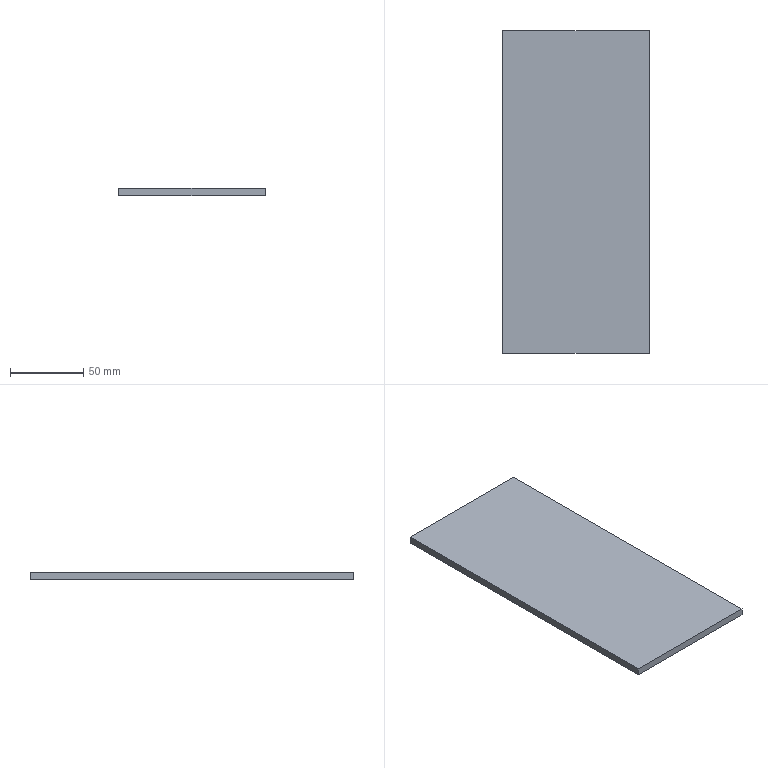Part | SolidWorks | features Extrusion 1 | 1 solid | 6 faces | box 100 x 220 x 5 mm | volume 110000 mm3 | plane 6
STEP:
#1=CARTESIAN_POINT('',(50.,-110.,0.));
#2=VERTEX_POINT('',#1);
#3=CARTESIAN_POINT('',(50.,110.,0.));
#4=VERTEX_POINT('',#3);
#5=CARTESIAN_POINT('',(50.,110.,0.));
#6=DIRECTION('',(0.,1.,0.));
#7=VECTOR('',#6,1000.);
#8=LINE('',#5,#7);
#9=EDGE_CURVE('',#2,#4,#8,.T.);
#10=ORIENTED_EDGE('',*,*,#9,.T.);
#11=CARTESIAN_POINT('',(50.,110.,5.));
#12=VERTEX_POINT('',#11);
#13=CARTESIAN_POINT('',(50.,110.,5.));
#14=DIRECTION('',(0.,0.,-1.));
#15=VECTOR('',#14,1000.);
#16=LINE('',#13,#15);
#17=EDGE_CURVE('',#12,#4,#16,.T.);
#18=ORIENTED_EDGE('',*,*,#17,.F.);
#19=CARTESIAN_POINT('',(50.,-110.,5.));
#20=VERTEX_POINT('',#19);
#21=CARTESIAN_POINT('',(50.,110.,5.));
#22=DIRECTION('',(0.,1.,0.));
#23=VECTOR('',#22,1000.);
#24=LINE('',#21,#23);
#25=EDGE_CURVE('',#20,#12,#24,.T.);
#26=ORIENTED_EDGE('',*,*,#25,.F.);
#27=CARTESIAN_POINT('',(50.,-110.,5.));
#28=DIRECTION('',(0.,0.,-1.));
#29=VECTOR('',#28,1000.);
#30=LINE('',#27,#29);
#31=EDGE_CURVE('',#20,#2,#30,.T.);
#32=ORIENTED_EDGE('',*,*,#31,.T.);
#33=EDGE_LOOP('',(#10,#18,#26,#32));
#34=FACE_OUTER_BOUND('',#33,.T.);
#35=CARTESIAN_POINT('',(50.,110.,5.));
#36=DIRECTION('',(-1.,0.,0.));
#37=DIRECTION('',(0.,-1.,0.));
#38=AXIS2_PLACEMENT_3D('',#35,#36,#37);
#39=PLANE('',#38);
#40=ADVANCED_FACE('',(#34),#39,.F.);
#41=CARTESIAN_POINT('',(-50.,110.,0.));
#42=VERTEX_POINT('',#41);
#43=CARTESIAN_POINT('',(-50.,110.,0.));
#44=DIRECTION('',(-1.,0.,0.));
#45=VECTOR('',#44,1000.);
#46=LINE('',#43,#45);
#47=EDGE_CURVE('',#4,#42,#46,.T.);
#48=ORIENTED_EDGE('',*,*,#47,.T.);
#49=CARTESIAN_POINT('',(-50.,110.,5.));
#50=VERTEX_POINT('',#49);
#51=CARTESIAN_POINT('',(-50.,110.,5.));
#52=DIRECTION('',(0.,0.,-1.));
#53=VECTOR('',#52,1000.);
#54=LINE('',#51,#53);
#55=EDGE_CURVE('',#50,#42,#54,.T.);
#56=ORIENTED_EDGE('',*,*,#55,.F.);
#57=CARTESIAN_POINT('',(-50.,110.,5.));
#58=DIRECTION('',(-1.,0.,0.));
#59=VECTOR('',#58,1000.);
#60=LINE('',#57,#59);
#61=EDGE_CURVE('',#12,#50,#60,.T.);
#62=ORIENTED_EDGE('',*,*,#61,.F.);
#63=ORIENTED_EDGE('',*,*,#17,.T.);
#64=EDGE_LOOP('',(#48,#56,#62,#63));
#65=FACE_OUTER_BOUND('',#64,.T.);
#66=CARTESIAN_POINT('',(-50.,110.,5.));
#67=DIRECTION('',(0.,-1.,0.));
#68=DIRECTION('',(0.,0.,-1.));
#69=AXIS2_PLACEMENT_3D('',#66,#67,#68);
#70=PLANE('',#69);
#71=ADVANCED_FACE('',(#65),#70,.F.);
#72=CARTESIAN_POINT('',(-50.,-110.,0.));
#73=VERTEX_POINT('',#72);
#74=CARTESIAN_POINT('',(-50.,110.,0.));
#75=DIRECTION('',(0.,-1.,0.));
#76=VECTOR('',#75,1000.);
#77=LINE('',#74,#76);
#78=EDGE_CURVE('',#42,#73,#77,.T.);
#79=ORIENTED_EDGE('',*,*,#78,.T.);
#80=CARTESIAN_POINT('',(-50.,-110.,5.));
#81=VERTEX_POINT('',#80);
#82=CARTESIAN_POINT('',(-50.,-110.,5.));
#83=DIRECTION('',(0.,0.,-1.));
#84=VECTOR('',#83,1000.);
#85=LINE('',#82,#84);
#86=EDGE_CURVE('',#81,#73,#85,.T.);
#87=ORIENTED_EDGE('',*,*,#86,.F.);
#88=CARTESIAN_POINT('',(-50.,110.,5.));
#89=DIRECTION('',(0.,-1.,0.));
#90=VECTOR('',#89,1000.);
#91=LINE('',#88,#90);
#92=EDGE_CURVE('',#50,#81,#91,.T.);
#93=ORIENTED_EDGE('',*,*,#92,.F.);
#94=ORIENTED_EDGE('',*,*,#55,.T.);
#95=EDGE_LOOP('',(#79,#87,#93,#94));
#96=FACE_OUTER_BOUND('',#95,.T.);
#97=CARTESIAN_POINT('',(-50.,110.,5.));
#98=DIRECTION('',(1.,0.,0.));
#99=DIRECTION('',(0.,1.,0.));
#100=AXIS2_PLACEMENT_3D('',#97,#98,#99);
#101=PLANE('',#100);
#102=ADVANCED_FACE('',(#96),#101,.F.);
#103=CARTESIAN_POINT('',(-50.,-110.,0.));
#104=DIRECTION('',(1.,0.,0.));
#105=VECTOR('',#104,1000.);
#106=LINE('',#103,#105);
#107=EDGE_CURVE('',#73,#2,#106,.T.);
#108=ORIENTED_EDGE('',*,*,#107,.T.);
#109=ORIENTED_EDGE('',*,*,#31,.F.);
#110=CARTESIAN_POINT('',(-50.,-110.,5.));
#111=DIRECTION('',(1.,0.,0.));
#112=VECTOR('',#111,1000.);
#113=LINE('',#110,#112);
#114=EDGE_CURVE('',#81,#20,#113,.T.);
#115=ORIENTED_EDGE('',*,*,#114,.F.);
#116=ORIENTED_EDGE('',*,*,#86,.T.);
#117=EDGE_LOOP('',(#108,#109,#115,#116));
#118=FACE_OUTER_BOUND('',#117,.T.);
#119=CARTESIAN_POINT('',(-50.,-110.,5.));
#120=DIRECTION('',(0.,1.,0.));
#121=DIRECTION('',(0.,0.,1.));
#122=AXIS2_PLACEMENT_3D('',#119,#120,#121);
#123=PLANE('',#122);
#124=ADVANCED_FACE('',(#118),#123,.F.);
#125=ORIENTED_EDGE('',*,*,#25,.T.);
#126=ORIENTED_EDGE('',*,*,#61,.T.);
#127=ORIENTED_EDGE('',*,*,#92,.T.);
#128=ORIENTED_EDGE('',*,*,#114,.T.);
#129=EDGE_LOOP('',(#125,#126,#127,#128));
#130=FACE_OUTER_BOUND('',#129,.T.);
#131=CARTESIAN_POINT('',(0.,0.,5.));
#132=DIRECTION('',(0.,0.,1.));
#133=DIRECTION('',(1.,0.,0.));
#134=AXIS2_PLACEMENT_3D('',#131,#132,#133);
#135=PLANE('',#134);
#136=ADVANCED_FACE('',(#130),#135,.T.);
#137=ORIENTED_EDGE('',*,*,#9,.F.);
#138=ORIENTED_EDGE('',*,*,#107,.F.);
#139=ORIENTED_EDGE('',*,*,#78,.F.);
#140=ORIENTED_EDGE('',*,*,#47,.F.);
#141=EDGE_LOOP('',(#137,#138,#139,#140));
#142=FACE_OUTER_BOUND('',#141,.T.);
#143=CARTESIAN_POINT('',(0.,0.,0.));
#144=DIRECTION('',(0.,0.,1.));
#145=DIRECTION('',(1.,0.,0.));
#146=AXIS2_PLACEMENT_3D('',#143,#144,#145);
#147=PLANE('',#146);
#148=ADVANCED_FACE('',(#142),#147,.F.);
#149=CLOSED_SHELL('',(#40,#71,#102,#124,#136,#148));
#150=MANIFOLD_SOLID_BREP('',#149);
#151=CARTESIAN_POINT('',(0.,0.,0.));
#152=DIRECTION('',(0.,0.,1.));
#153=DIRECTION('',(1.,0.,0.));
#154=AXIS2_PLACEMENT_3D('',#151,#152,#153);
#155=(LENGTH_UNIT()NAMED_UNIT(*)SI_UNIT(.MILLI.,.METRE.));
#156=UNCERTAINTY_MEASURE_WITH_UNIT(LENGTH_MEASURE(0.00001),#155,'','');
#157=(NAMED_UNIT(*)PLANE_ANGLE_UNIT()SI_UNIT($,.RADIAN.));
#158=(NAMED_UNIT(*)SI_UNIT($,.STERADIAN.)SOLID_ANGLE_UNIT());
#159=(GEOMETRIC_REPRESENTATION_CONTEXT(3)GLOBAL_UNCERTAINTY_ASSIGNED_CONTEXT((#156))GLOBAL_UNIT_ASSIGNED_CONTEXT((#155,#157,#158))REPRESENTATION_CONTEXT('',''));
#160=ADVANCED_BREP_SHAPE_REPRESENTATION('',(#150,#154),#159);